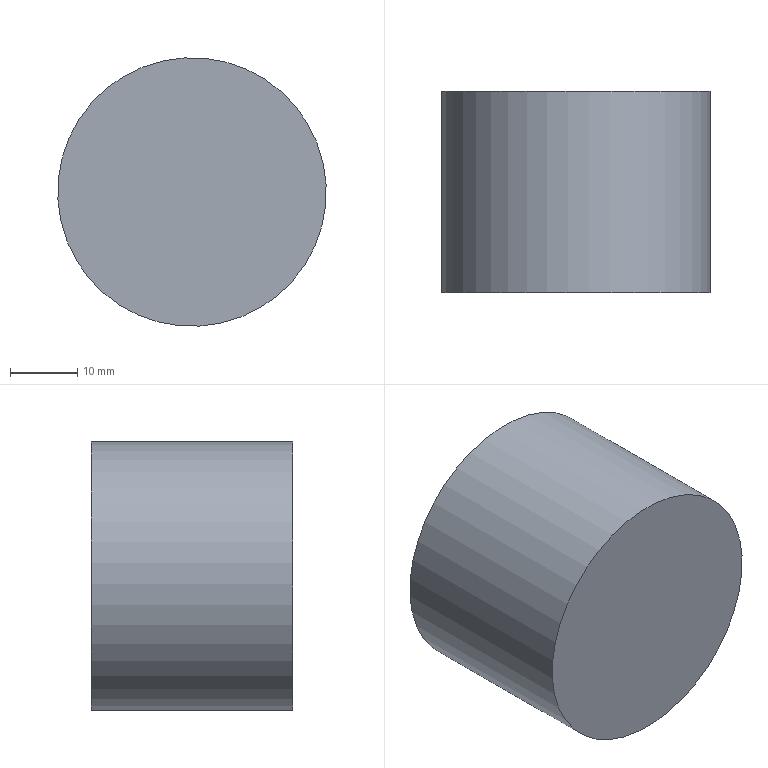Part | STEP file | a-hp_225_37-140_3_0_06 | 1 solid | 3 faces | box 40 x 30 x 40 mm | volume 37699 mm3 | plane 2 | cylinder 1 | commonest cylinder face diameters 40 x1
STEP:
#1=CARTESIAN_POINT('',(73.719,130.,82.036));
#2=VERTEX_POINT('',#1);
#3=CARTESIAN_POINT('',(78.,130.,62.5));
#4=DIRECTION('',(0.,1.,0.));
#5=DIRECTION('',(0.214,0.,-0.9768));
#6=AXIS2_PLACEMENT_3D('',#3,#4,#5);
#7=CIRCLE('',#6,20.);
#8=EDGE_CURVE('',#2,#2,#7,.T.);
#9=ORIENTED_EDGE('',*,*,#8,.F.);
#10=CARTESIAN_POINT('',(73.719,100.,82.036));
#11=VERTEX_POINT('',#10);
#12=CARTESIAN_POINT('',(73.719,100.,82.036));
#13=DIRECTION('',(0.,-1.,0.));
#14=VECTOR('',#13,20.);
#15=LINE('',#12,#14);
#16=EDGE_CURVE('',#2,#11,#15,.T.);
#17=ORIENTED_EDGE('',*,*,#16,.T.);
#18=CARTESIAN_POINT('',(78.,100.,62.5));
#19=DIRECTION('',(0.,-1.,0.));
#20=DIRECTION('',(0.214,0.,-0.9768));
#21=AXIS2_PLACEMENT_3D('',#18,#19,#20);
#22=CIRCLE('',#21,20.);
#23=EDGE_CURVE('',#11,#11,#22,.T.);
#24=ORIENTED_EDGE('',*,*,#23,.F.);
#25=ORIENTED_EDGE('',*,*,#16,.F.);
#26=EDGE_LOOP('',(#9,#17,#24,#25));
#27=FACE_OUTER_BOUND('',#26,.T.);
#28=CARTESIAN_POINT('',(78.,100.,62.5));
#29=DIRECTION('',(0.,-1.,0.));
#30=DIRECTION('',(0.214,0.,-0.9768));
#31=AXIS2_PLACEMENT_3D('',#28,#29,#30);
#32=CYLINDRICAL_SURFACE('',#31,20.);
#33=ADVANCED_FACE('',(#27),#32,.T.);
#34=ORIENTED_EDGE('',*,*,#23,.T.);
#35=EDGE_LOOP('',(#34));
#36=FACE_OUTER_BOUND('',#35,.T.);
#37=CARTESIAN_POINT('',(78.,100.,62.5));
#38=DIRECTION('',(0.,1.,0.));
#39=DIRECTION('',(-0.214,0.,0.9768));
#40=AXIS2_PLACEMENT_3D('',#37,#38,#39);
#41=PLANE('',#40);
#42=ADVANCED_FACE('',(#36),#41,.F.);
#43=ORIENTED_EDGE('',*,*,#8,.T.);
#44=EDGE_LOOP('',(#43));
#45=FACE_OUTER_BOUND('',#44,.T.);
#46=CARTESIAN_POINT('',(78.,130.,62.5));
#47=DIRECTION('',(0.,1.,0.));
#48=DIRECTION('',(-0.214,0.,0.9768));
#49=AXIS2_PLACEMENT_3D('',#46,#47,#48);
#50=PLANE('',#49);
#51=ADVANCED_FACE('',(#45),#50,.T.);
#52=CLOSED_SHELL('',(#33,#42,#51));
#53=MANIFOLD_SOLID_BREP('',#52);
#54=(LENGTH_UNIT()NAMED_UNIT(*)SI_UNIT(.MILLI.,.METRE.));
#55=UNCERTAINTY_MEASURE_WITH_UNIT(LENGTH_MEASURE(0.01),#54,'','');
#56=(NAMED_UNIT(*)PLANE_ANGLE_UNIT()SI_UNIT($,.RADIAN.));
#57=(NAMED_UNIT(*)SI_UNIT($,.STERADIAN.)SOLID_ANGLE_UNIT());
#58=(GEOMETRIC_REPRESENTATION_CONTEXT(3)GLOBAL_UNCERTAINTY_ASSIGNED_CONTEXT((#55))GLOBAL_UNIT_ASSIGNED_CONTEXT((#54,#56,#57))REPRESENTATION_CONTEXT('',''));
#59=ADVANCED_BREP_SHAPE_REPRESENTATION('',(#53),#58);